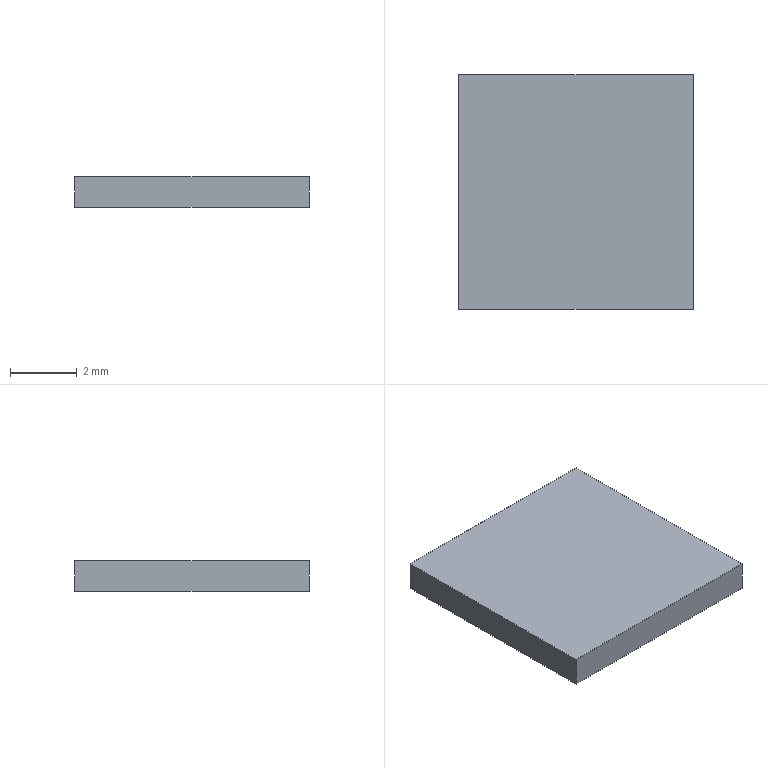Part | Creo | 1 solid | 6 faces | box 7.035 x 7.035 x 0.9 mm | volume 44.542 mm3 | plane 6
STEP:
#1=CARTESIAN_POINT('',(0.,0.,0.));
#2=DIRECTION('',(0.,0.,1.));
#3=DIRECTION('',(1.,0.,0.));
#4=AXIS2_PLACEMENT_3D('',#1,#2,#3);
#5=CARTESIAN_POINT('',(-3.518,-3.518,0.));
#6=VERTEX_POINT('',#5);
#7=CARTESIAN_POINT('',(3.518,-3.518,0.));
#8=VERTEX_POINT('',#7);
#9=CARTESIAN_POINT('',(-3.518,-3.518,0.));
#10=DIRECTION('',(1.,0.,0.));
#11=VECTOR('',#10,7.035);
#12=LINE('',#9,#11);
#13=EDGE_CURVE('',#6,#8,#12,.T.);
#14=ORIENTED_EDGE('',*,*,#13,.T.);
#15=CARTESIAN_POINT('',(3.518,3.518,0.));
#16=VERTEX_POINT('',#15);
#17=CARTESIAN_POINT('',(3.518,-3.518,0.));
#18=DIRECTION('',(0.,1.,0.));
#19=VECTOR('',#18,7.035);
#20=LINE('',#17,#19);
#21=EDGE_CURVE('',#8,#16,#20,.T.);
#22=ORIENTED_EDGE('',*,*,#21,.T.);
#23=CARTESIAN_POINT('',(-3.518,3.518,0.));
#24=VERTEX_POINT('',#23);
#25=CARTESIAN_POINT('',(3.518,3.518,0.));
#26=DIRECTION('',(-1.,0.,0.));
#27=VECTOR('',#26,7.035);
#28=LINE('',#25,#27);
#29=EDGE_CURVE('',#16,#24,#28,.T.);
#30=ORIENTED_EDGE('',*,*,#29,.T.);
#31=CARTESIAN_POINT('',(-3.518,3.518,0.));
#32=DIRECTION('',(0.,-1.,0.));
#33=VECTOR('',#32,7.035);
#34=LINE('',#31,#33);
#35=EDGE_CURVE('',#24,#6,#34,.T.);
#36=ORIENTED_EDGE('',*,*,#35,.T.);
#37=EDGE_LOOP('',(#14,#22,#30,#36));
#38=FACE_OUTER_BOUND('',#37,.F.);
#39=CARTESIAN_POINT('',(0.,0.,0.));
#40=DIRECTION('',(0.,0.,1.));
#41=DIRECTION('',(1.,0.,0.));
#42=AXIS2_PLACEMENT_3D('',#39,#40,#41);
#43=PLANE('',#42);
#44=ADVANCED_FACE('',(#38),#43,.F.);
#45=ORIENTED_EDGE('',*,*,#13,.F.);
#46=CARTESIAN_POINT('',(-3.518,-3.518,0.9));
#47=VERTEX_POINT('',#46);
#48=CARTESIAN_POINT('',(-3.518,-3.518,0.));
#49=DIRECTION('',(0.,0.,1.));
#50=VECTOR('',#49,0.9);
#51=LINE('',#48,#50);
#52=EDGE_CURVE('',#6,#47,#51,.T.);
#53=ORIENTED_EDGE('',*,*,#52,.T.);
#54=CARTESIAN_POINT('',(3.518,-3.518,0.9));
#55=VERTEX_POINT('',#54);
#56=CARTESIAN_POINT('',(-3.518,-3.518,0.9));
#57=DIRECTION('',(1.,0.,0.));
#58=VECTOR('',#57,7.035);
#59=LINE('',#56,#58);
#60=EDGE_CURVE('',#47,#55,#59,.T.);
#61=ORIENTED_EDGE('',*,*,#60,.T.);
#62=CARTESIAN_POINT('',(3.518,-3.518,0.));
#63=DIRECTION('',(0.,0.,1.));
#64=VECTOR('',#63,0.9);
#65=LINE('',#62,#64);
#66=EDGE_CURVE('',#8,#55,#65,.T.);
#67=ORIENTED_EDGE('',*,*,#66,.F.);
#68=EDGE_LOOP('',(#45,#53,#61,#67));
#69=FACE_OUTER_BOUND('',#68,.F.);
#70=CARTESIAN_POINT('',(-3.518,-3.518,0.));
#71=DIRECTION('',(0.,-1.,0.));
#72=DIRECTION('',(1.,0.,0.));
#73=AXIS2_PLACEMENT_3D('',#70,#71,#72);
#74=PLANE('',#73);
#75=ADVANCED_FACE('',(#69),#74,.T.);
#76=ORIENTED_EDGE('',*,*,#35,.F.);
#77=CARTESIAN_POINT('',(-3.518,3.518,0.9));
#78=VERTEX_POINT('',#77);
#79=CARTESIAN_POINT('',(-3.518,3.518,0.));
#80=DIRECTION('',(0.,0.,1.));
#81=VECTOR('',#80,0.9);
#82=LINE('',#79,#81);
#83=EDGE_CURVE('',#24,#78,#82,.T.);
#84=ORIENTED_EDGE('',*,*,#83,.T.);
#85=CARTESIAN_POINT('',(-3.518,3.518,0.9));
#86=DIRECTION('',(0.,-1.,0.));
#87=VECTOR('',#86,7.035);
#88=LINE('',#85,#87);
#89=EDGE_CURVE('',#78,#47,#88,.T.);
#90=ORIENTED_EDGE('',*,*,#89,.T.);
#91=ORIENTED_EDGE('',*,*,#52,.F.);
#92=EDGE_LOOP('',(#76,#84,#90,#91));
#93=FACE_OUTER_BOUND('',#92,.F.);
#94=CARTESIAN_POINT('',(-3.518,3.518,0.));
#95=DIRECTION('',(-1.,0.,0.));
#96=DIRECTION('',(0.,-1.,0.));
#97=AXIS2_PLACEMENT_3D('',#94,#95,#96);
#98=PLANE('',#97);
#99=ADVANCED_FACE('',(#93),#98,.T.);
#100=ORIENTED_EDGE('',*,*,#29,.F.);
#101=CARTESIAN_POINT('',(3.518,3.518,0.9));
#102=VERTEX_POINT('',#101);
#103=CARTESIAN_POINT('',(3.518,3.518,0.));
#104=DIRECTION('',(0.,0.,1.));
#105=VECTOR('',#104,0.9);
#106=LINE('',#103,#105);
#107=EDGE_CURVE('',#16,#102,#106,.T.);
#108=ORIENTED_EDGE('',*,*,#107,.T.);
#109=CARTESIAN_POINT('',(3.518,3.518,0.9));
#110=DIRECTION('',(-1.,0.,0.));
#111=VECTOR('',#110,7.035);
#112=LINE('',#109,#111);
#113=EDGE_CURVE('',#102,#78,#112,.T.);
#114=ORIENTED_EDGE('',*,*,#113,.T.);
#115=ORIENTED_EDGE('',*,*,#83,.F.);
#116=EDGE_LOOP('',(#100,#108,#114,#115));
#117=FACE_OUTER_BOUND('',#116,.F.);
#118=CARTESIAN_POINT('',(3.518,3.518,0.));
#119=DIRECTION('',(0.,1.,0.));
#120=DIRECTION('',(-1.,0.,0.));
#121=AXIS2_PLACEMENT_3D('',#118,#119,#120);
#122=PLANE('',#121);
#123=ADVANCED_FACE('',(#117),#122,.T.);
#124=ORIENTED_EDGE('',*,*,#21,.F.);
#125=ORIENTED_EDGE('',*,*,#66,.T.);
#126=CARTESIAN_POINT('',(3.518,-3.518,0.9));
#127=DIRECTION('',(0.,1.,0.));
#128=VECTOR('',#127,7.035);
#129=LINE('',#126,#128);
#130=EDGE_CURVE('',#55,#102,#129,.T.);
#131=ORIENTED_EDGE('',*,*,#130,.T.);
#132=ORIENTED_EDGE('',*,*,#107,.F.);
#133=EDGE_LOOP('',(#124,#125,#131,#132));
#134=FACE_OUTER_BOUND('',#133,.F.);
#135=CARTESIAN_POINT('',(3.518,-3.518,0.));
#136=DIRECTION('',(1.,0.,0.));
#137=DIRECTION('',(0.,1.,0.));
#138=AXIS2_PLACEMENT_3D('',#135,#136,#137);
#139=PLANE('',#138);
#140=ADVANCED_FACE('',(#134),#139,.T.);
#141=ORIENTED_EDGE('',*,*,#60,.F.);
#142=ORIENTED_EDGE('',*,*,#89,.F.);
#143=ORIENTED_EDGE('',*,*,#113,.F.);
#144=ORIENTED_EDGE('',*,*,#130,.F.);
#145=EDGE_LOOP('',(#141,#142,#143,#144));
#146=FACE_OUTER_BOUND('',#145,.F.);
#147=CARTESIAN_POINT('',(0.,0.,0.9));
#148=DIRECTION('',(0.,0.,1.));
#149=DIRECTION('',(1.,0.,0.));
#150=AXIS2_PLACEMENT_3D('',#147,#148,#149);
#151=PLANE('',#150);
#152=ADVANCED_FACE('',(#146),#151,.T.);
#153=CLOSED_SHELL('',(#44,#75,#99,#123,#140,#152));
#154=MANIFOLD_SOLID_BREP('',#153);
#155=(LENGTH_UNIT()NAMED_UNIT(*)SI_UNIT(.MILLI.,.METRE.));
#156=UNCERTAINTY_MEASURE_WITH_UNIT(LENGTH_MEASURE(0.0009989),#155,'','');
#157=(NAMED_UNIT(*)PLANE_ANGLE_UNIT()SI_UNIT($,.RADIAN.));
#158=PLANE_ANGLE_MEASURE_WITH_UNIT(PLANE_ANGLE_MEASURE(0.01745),#157);
#159=(CONVERSION_BASED_UNIT('DEGREE',#158)NAMED_UNIT(*)PLANE_ANGLE_UNIT());
#160=(NAMED_UNIT(*)SI_UNIT($,.STERADIAN.)SOLID_ANGLE_UNIT());
#161=(GEOMETRIC_REPRESENTATION_CONTEXT(3)GLOBAL_UNCERTAINTY_ASSIGNED_CONTEXT((#156))GLOBAL_UNIT_ASSIGNED_CONTEXT((#155,#159,#160))REPRESENTATION_CONTEXT('',''));
#162=ADVANCED_BREP_SHAPE_REPRESENTATION('',(#4,#154),#161);